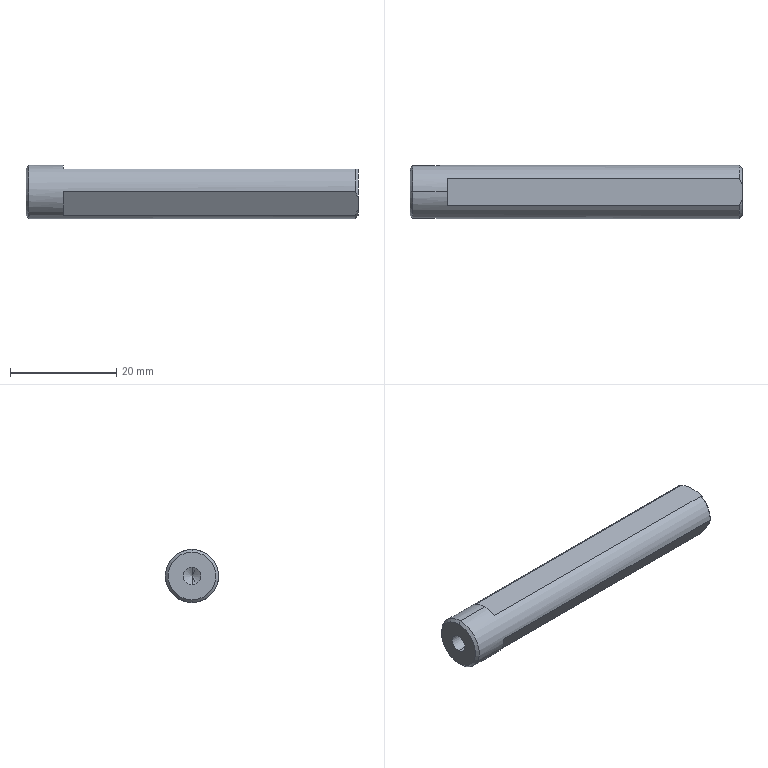Part | SolidWorks | features Chamfer 1, CirPattern 1, Extrusion 1, HoleWzd 1, ICE 1 | 1 solid | 19 faces | box 62.5 x 10 x 10 mm | volume 4365 mm3 | plane 8 | cone 7 | cylinder 4 | commonest cylinder face diameters 3.3 x2 10 x2
STEP:
#1=CARTESIAN_POINT('',(15.5,0.,-1.65));
#2=VERTEX_POINT('',#1);
#3=CARTESIAN_POINT('',(15.5,0.,1.65));
#4=VERTEX_POINT('',#3);
#5=CARTESIAN_POINT('',(15.5,0.,0.));
#6=DIRECTION('',(-1.,0.,0.));
#7=DIRECTION('',(0.,0.,1.));
#8=AXIS2_PLACEMENT_3D('',#5,#6,#7);
#9=CIRCLE('',#8,1.65);
#10=EDGE_CURVE('',#2,#4,#9,.T.);
#11=ORIENTED_EDGE('',*,*,#10,.F.);
#12=CARTESIAN_POINT('',(0.,0.,-1.65));
#13=VERTEX_POINT('',#12);
#14=CARTESIAN_POINT('',(0.,0.,-1.65));
#15=DIRECTION('',(-1.,0.,0.));
#16=VECTOR('',#15,1000.);
#17=LINE('',#14,#16);
#18=EDGE_CURVE('',#2,#13,#17,.T.);
#19=ORIENTED_EDGE('',*,*,#18,.T.);
#20=CARTESIAN_POINT('',(0.,0.,1.65));
#21=VERTEX_POINT('',#20);
#22=CARTESIAN_POINT('',(0.,0.,0.));
#23=DIRECTION('',(-1.,0.,0.));
#24=DIRECTION('',(0.,0.,1.));
#25=AXIS2_PLACEMENT_3D('',#22,#23,#24);
#26=CIRCLE('',#25,1.65);
#27=EDGE_CURVE('',#13,#21,#26,.T.);
#28=ORIENTED_EDGE('',*,*,#27,.T.);
#29=CARTESIAN_POINT('',(0.,0.,1.65));
#30=DIRECTION('',(-1.,0.,0.));
#31=VECTOR('',#30,1000.);
#32=LINE('',#29,#31);
#33=EDGE_CURVE('',#4,#21,#32,.T.);
#34=ORIENTED_EDGE('',*,*,#33,.F.);
#35=EDGE_LOOP('',(#11,#19,#28,#34));
#36=FACE_OUTER_BOUND('',#35,.T.);
#37=CARTESIAN_POINT('',(0.,0.,0.));
#38=DIRECTION('',(-1.,0.,0.));
#39=DIRECTION('',(0.,0.,1.));
#40=AXIS2_PLACEMENT_3D('',#37,#38,#39);
#41=CYLINDRICAL_SURFACE('',#40,1.65);
#42=ADVANCED_FACE('',(#36),#41,.F.);
#43=CARTESIAN_POINT('',(16.491,0.,0.));
#44=VERTEX_POINT('',#43);
#45=CARTESIAN_POINT('',(15.5,0.,1.65));
#46=DIRECTION('',(-0.515,0.,0.8572));
#47=VECTOR('',#46,1000.);
#48=LINE('',#45,#47);
#49=EDGE_CURVE('',#44,#4,#48,.T.);
#50=ORIENTED_EDGE('',*,*,#49,.F.);
#51=CARTESIAN_POINT('',(15.5,0.,-1.65));
#52=DIRECTION('',(-0.515,0.,-0.8572));
#53=VECTOR('',#52,1000.);
#54=LINE('',#51,#53);
#55=EDGE_CURVE('',#44,#2,#54,.T.);
#56=ORIENTED_EDGE('',*,*,#55,.T.);
#57=ORIENTED_EDGE('',*,*,#10,.T.);
#58=EDGE_LOOP('',(#50,#56,#57));
#59=FACE_OUTER_BOUND('',#58,.T.);
#60=CARTESIAN_POINT('',(15.5,0.,0.));
#61=DIRECTION('',(-1.,0.,0.));
#62=DIRECTION('',(0.,0.,1.));
#63=AXIS2_PLACEMENT_3D('',#60,#61,#62);
#64=CONICAL_SURFACE('',#63,1.65,1.03);
#65=ADVANCED_FACE('',(#59),#64,.F.);
#66=CARTESIAN_POINT('',(0.,0.,4.5));
#67=VERTEX_POINT('',#66);
#68=CARTESIAN_POINT('',(0.,0.,-4.5));
#69=VERTEX_POINT('',#68);
#70=CARTESIAN_POINT('',(0.,0.,0.));
#71=DIRECTION('',(-1.,0.,0.));
#72=DIRECTION('',(0.,0.,-1.));
#73=AXIS2_PLACEMENT_3D('',#70,#71,#72);
#74=CIRCLE('',#73,4.5);
#75=EDGE_CURVE('',#67,#69,#74,.T.);
#76=ORIENTED_EDGE('',*,*,#75,.F.);
#77=CARTESIAN_POINT('',(0.5,0.,5.));
#78=VERTEX_POINT('',#77);
#79=CARTESIAN_POINT('',(0.5,0.,5.));
#80=DIRECTION('',(0.7071,0.,0.7071));
#81=VECTOR('',#80,1000.);
#82=LINE('',#79,#81);
#83=EDGE_CURVE('',#67,#78,#82,.T.);
#84=ORIENTED_EDGE('',*,*,#83,.T.);
#85=CARTESIAN_POINT('',(0.5,0.,-5.));
#86=VERTEX_POINT('',#85);
#87=CARTESIAN_POINT('',(0.5,0.,0.));
#88=DIRECTION('',(1.,0.,0.));
#89=DIRECTION('',(0.,0.,-1.));
#90=AXIS2_PLACEMENT_3D('',#87,#88,#89);
#91=CIRCLE('',#90,5.);
#92=EDGE_CURVE('',#86,#78,#91,.T.);
#93=ORIENTED_EDGE('',*,*,#92,.F.);
#94=CARTESIAN_POINT('',(0.5,0.,-5.));
#95=DIRECTION('',(0.7071,0.,-0.7071));
#96=VECTOR('',#95,1000.);
#97=LINE('',#94,#96);
#98=EDGE_CURVE('',#69,#86,#97,.T.);
#99=ORIENTED_EDGE('',*,*,#98,.F.);
#100=EDGE_LOOP('',(#76,#84,#93,#99));
#101=FACE_OUTER_BOUND('',#100,.T.);
#102=CARTESIAN_POINT('',(0.5,0.,0.));
#103=DIRECTION('',(1.,0.,0.));
#104=DIRECTION('',(0.,0.,-1.));
#105=AXIS2_PLACEMENT_3D('',#102,#103,#104);
#106=CONICAL_SURFACE('',#105,5.,0.7854);
#107=ADVANCED_FACE('',(#101),#106,.T.);
#108=CARTESIAN_POINT('',(62.,2.448,-4.36));
#109=VERTEX_POINT('',#108);
#110=CARTESIAN_POINT('',(62.,0.,-5.));
#111=VERTEX_POINT('',#110);
#112=CARTESIAN_POINT('',(62.,0.,0.));
#113=DIRECTION('',(-1.,0.,0.));
#114=DIRECTION('',(0.,0.,-1.));
#115=AXIS2_PLACEMENT_3D('',#112,#113,#114);
#116=CIRCLE('',#115,5.);
#117=EDGE_CURVE('',#109,#111,#116,.T.);
#118=ORIENTED_EDGE('',*,*,#117,.T.);
#119=CARTESIAN_POINT('',(62.5,0.,-5.));
#120=DIRECTION('',(-1.,0.,0.));
#121=VECTOR('',#120,1000.);
#122=LINE('',#119,#121);
#123=EDGE_CURVE('',#111,#86,#122,.T.);
#124=ORIENTED_EDGE('',*,*,#123,.T.);
#125=ORIENTED_EDGE('',*,*,#92,.T.);
#126=CARTESIAN_POINT('',(7.,0.,5.));
#127=VERTEX_POINT('',#126);
#128=CARTESIAN_POINT('',(62.5,0.,5.));
#129=DIRECTION('',(-1.,0.,0.));
#130=VECTOR('',#129,1000.);
#131=LINE('',#128,#130);
#132=EDGE_CURVE('',#127,#78,#131,.T.);
#133=ORIENTED_EDGE('',*,*,#132,.F.);
#134=CARTESIAN_POINT('',(7.,2.551,4.3));
#135=VERTEX_POINT('',#134);
#136=CARTESIAN_POINT('',(7.,0.,0.));
#137=DIRECTION('',(1.,0.,0.));
#138=DIRECTION('',(0.,0.,-1.));
#139=AXIS2_PLACEMENT_3D('',#136,#137,#138);
#140=CIRCLE('',#139,5.);
#141=EDGE_CURVE('',#135,#127,#140,.T.);
#142=ORIENTED_EDGE('',*,*,#141,.F.);
#143=CARTESIAN_POINT('',(62.,2.551,4.3));
#144=VERTEX_POINT('',#143);
#145=CARTESIAN_POINT('',(62.5,2.551,4.3));
#146=DIRECTION('',(1.,0.,0.));
#147=VECTOR('',#146,1000.);
#148=LINE('',#145,#147);
#149=EDGE_CURVE('',#135,#144,#148,.T.);
#150=ORIENTED_EDGE('',*,*,#149,.T.);
#151=CARTESIAN_POINT('',(62.,5.,0.05964));
#152=VERTEX_POINT('',#151);
#153=CARTESIAN_POINT('',(62.,0.,0.));
#154=DIRECTION('',(-1.,0.,0.));
#155=DIRECTION('',(0.,0.,-1.));
#156=AXIS2_PLACEMENT_3D('',#153,#154,#155);
#157=CIRCLE('',#156,5.);
#158=EDGE_CURVE('',#144,#152,#157,.T.);
#159=ORIENTED_EDGE('',*,*,#158,.T.);
#160=CARTESIAN_POINT('',(7.,5.,0.05964));
#161=VERTEX_POINT('',#160);
#162=CARTESIAN_POINT('',(62.5,5.,0.05964));
#163=DIRECTION('',(-1.,0.,0.));
#164=VECTOR('',#163,1000.);
#165=LINE('',#162,#164);
#166=EDGE_CURVE('',#152,#161,#165,.T.);
#167=ORIENTED_EDGE('',*,*,#166,.T.);
#168=CARTESIAN_POINT('',(7.,2.448,-4.36));
#169=VERTEX_POINT('',#168);
#170=CARTESIAN_POINT('',(7.,0.,0.));
#171=DIRECTION('',(1.,0.,0.));
#172=DIRECTION('',(0.,0.,-1.));
#173=AXIS2_PLACEMENT_3D('',#170,#171,#172);
#174=CIRCLE('',#173,5.);
#175=EDGE_CURVE('',#169,#161,#174,.T.);
#176=ORIENTED_EDGE('',*,*,#175,.F.);
#177=CARTESIAN_POINT('',(62.5,2.448,-4.36));
#178=DIRECTION('',(1.,0.,0.));
#179=VECTOR('',#178,1000.);
#180=LINE('',#177,#179);
#181=EDGE_CURVE('',#169,#109,#180,.T.);
#182=ORIENTED_EDGE('',*,*,#181,.T.);
#183=EDGE_LOOP('',(#118,#124,#125,#133,#142,#150,#159,#167,#176,#182));
#184=FACE_OUTER_BOUND('',#183,.T.);
#185=CARTESIAN_POINT('',(62.5,0.,0.));
#186=DIRECTION('',(-1.,0.,0.));
#187=DIRECTION('',(0.,0.,1.));
#188=AXIS2_PLACEMENT_3D('',#185,#186,#187);
#189=CYLINDRICAL_SURFACE('',#188,5.);
#190=ADVANCED_FACE('',(#184),#189,.T.);
#191=CARTESIAN_POINT('',(62.,-2.448,-4.36));
#192=VERTEX_POINT('',#191);
#193=CARTESIAN_POINT('',(62.5,-3.061,-3.299));
#194=VERTEX_POINT('',#193);
#195=CARTESIAN_POINT('',(62.,-2.448,-4.36));
#196=CARTESIAN_POINT('',(62.201,-2.645,-4.019));
#197=CARTESIAN_POINT('',(62.374,-2.847,-3.668));
#198=CARTESIAN_POINT('',(62.5,-3.061,-3.299));
#199=B_SPLINE_CURVE_WITH_KNOTS('',3,(#195,#196,#197,#198),.UNSPECIFIED.,.F.,.F.,(4,4),(0.009242,0.01057),.UNSPECIFIED.);
#200=EDGE_CURVE('',#192,#194,#199,.T.);
#201=ORIENTED_EDGE('',*,*,#200,.F.);
#202=CARTESIAN_POINT('',(62.,0.,0.));
#203=DIRECTION('',(-1.,0.,0.));
#204=DIRECTION('',(0.,0.,-1.));
#205=AXIS2_PLACEMENT_3D('',#202,#203,#204);
#206=CIRCLE('',#205,5.);
#207=EDGE_CURVE('',#111,#192,#206,.T.);
#208=ORIENTED_EDGE('',*,*,#207,.F.);
#209=ORIENTED_EDGE('',*,*,#117,.F.);
#210=CARTESIAN_POINT('',(62.5,3.061,-3.299));
#211=VERTEX_POINT('',#210);
#212=CARTESIAN_POINT('',(62.5,3.061,-3.299));
#213=CARTESIAN_POINT('',(62.438,2.955,-3.482));
#214=CARTESIAN_POINT('',(62.362,2.85,-3.664));
#215=CARTESIAN_POINT('',(62.193,2.645,-4.018));
#216=CARTESIAN_POINT('',(62.1,2.546,-4.191));
#217=CARTESIAN_POINT('',(62.,2.448,-4.36));
#218=B_SPLINE_CURVE_WITH_KNOTS('',3,(#212,#213,#214,#215,#216,#217),.UNSPECIFIED.,.F.,.F.,(4,2,4),(0.01336,0.01402,0.01468),.UNSPECIFIED.);
#219=EDGE_CURVE('',#211,#109,#218,.T.);
#220=ORIENTED_EDGE('',*,*,#219,.F.);
#221=CARTESIAN_POINT('',(62.5,0.,0.));
#222=DIRECTION('',(1.,0.,0.));
#223=DIRECTION('',(0.,0.,-1.));
#224=AXIS2_PLACEMENT_3D('',#221,#222,#223);
#225=CIRCLE('',#224,4.5);
#226=EDGE_CURVE('',#194,#211,#225,.T.);
#227=ORIENTED_EDGE('',*,*,#226,.F.);
#228=EDGE_LOOP('',(#201,#208,#209,#220,#227));
#229=FACE_OUTER_BOUND('',#228,.T.);
#230=CARTESIAN_POINT('',(62.5,0.,0.));
#231=DIRECTION('',(-1.,0.,0.));
#232=DIRECTION('',(0.,0.,1.));
#233=AXIS2_PLACEMENT_3D('',#230,#231,#232);
#234=CONICAL_SURFACE('',#233,4.5,0.7854);
#235=ADVANCED_FACE('',(#229),#234,.T.);
#236=CARTESIAN_POINT('',(62.5,4.387,-1.001));
#237=VERTEX_POINT('',#236);
#238=CARTESIAN_POINT('',(62.,5.,0.05964));
#239=CARTESIAN_POINT('',(62.201,4.803,-0.2807));
#240=CARTESIAN_POINT('',(62.374,4.601,-0.6315));
#241=CARTESIAN_POINT('',(62.5,4.387,-1.001));
#242=B_SPLINE_CURVE_WITH_KNOTS('',3,(#238,#239,#240,#241),.UNSPECIFIED.,.F.,.F.,(4,4),(0.00934,0.01066),.UNSPECIFIED.);
#243=EDGE_CURVE('',#152,#237,#242,.T.);
#244=ORIENTED_EDGE('',*,*,#243,.F.);
#245=ORIENTED_EDGE('',*,*,#158,.F.);
#246=CARTESIAN_POINT('',(62.5,1.327,4.3));
#247=VERTEX_POINT('',#246);
#248=CARTESIAN_POINT('',(62.5,1.327,4.3));
#249=CARTESIAN_POINT('',(62.437,1.539,4.3));
#250=CARTESIAN_POINT('',(62.362,1.749,4.3));
#251=CARTESIAN_POINT('',(62.193,2.157,4.3));
#252=CARTESIAN_POINT('',(62.1,2.356,4.3));
#253=CARTESIAN_POINT('',(62.,2.551,4.3));
#254=B_SPLINE_CURVE_WITH_KNOTS('',3,(#248,#249,#250,#251,#252,#253),.UNSPECIFIED.,.F.,.F.,(4,2,4),(0.01372,0.01438,0.01504),.UNSPECIFIED.);
#255=EDGE_CURVE('',#247,#144,#254,.T.);
#256=ORIENTED_EDGE('',*,*,#255,.F.);
#257=CARTESIAN_POINT('',(62.5,0.,0.));
#258=DIRECTION('',(1.,0.,0.));
#259=DIRECTION('',(0.,0.,-1.));
#260=AXIS2_PLACEMENT_3D('',#257,#258,#259);
#261=CIRCLE('',#260,4.5);
#262=EDGE_CURVE('',#237,#247,#261,.T.);
#263=ORIENTED_EDGE('',*,*,#262,.F.);
#264=EDGE_LOOP('',(#244,#245,#256,#263));
#265=FACE_OUTER_BOUND('',#264,.T.);
#266=CARTESIAN_POINT('',(62.5,0.,0.));
#267=DIRECTION('',(-1.,0.,0.));
#268=DIRECTION('',(0.,0.,1.));
#269=AXIS2_PLACEMENT_3D('',#266,#267,#268);
#270=CONICAL_SURFACE('',#269,4.5,0.7854);
#271=ADVANCED_FACE('',(#265),#270,.T.);
#272=ORIENTED_EDGE('',*,*,#123,.F.);
#273=ORIENTED_EDGE('',*,*,#207,.T.);
#274=CARTESIAN_POINT('',(7.,-2.448,-4.36));
#275=VERTEX_POINT('',#274);
#276=CARTESIAN_POINT('',(62.5,-2.448,-4.36));
#277=DIRECTION('',(-1.,0.,0.));
#278=VECTOR('',#277,1000.);
#279=LINE('',#276,#278);
#280=EDGE_CURVE('',#192,#275,#279,.T.);
#281=ORIENTED_EDGE('',*,*,#280,.T.);
#282=CARTESIAN_POINT('',(7.,-5.,0.05964));
#283=VERTEX_POINT('',#282);
#284=CARTESIAN_POINT('',(7.,0.,0.));
#285=DIRECTION('',(1.,0.,0.));
#286=DIRECTION('',(0.,0.,-1.));
#287=AXIS2_PLACEMENT_3D('',#284,#285,#286);
#288=CIRCLE('',#287,5.);
#289=EDGE_CURVE('',#283,#275,#288,.T.);
#290=ORIENTED_EDGE('',*,*,#289,.F.);
#291=CARTESIAN_POINT('',(62.,-5.,0.05964));
#292=VERTEX_POINT('',#291);
#293=CARTESIAN_POINT('',(62.5,-5.,0.05964));
#294=DIRECTION('',(1.,0.,0.));
#295=VECTOR('',#294,1000.);
#296=LINE('',#293,#295);
#297=EDGE_CURVE('',#283,#292,#296,.T.);
#298=ORIENTED_EDGE('',*,*,#297,.T.);
#299=CARTESIAN_POINT('',(62.,-2.551,4.3));
#300=VERTEX_POINT('',#299);
#301=CARTESIAN_POINT('',(62.,0.,0.));
#302=DIRECTION('',(-1.,0.,0.));
#303=DIRECTION('',(0.,0.,-1.));
#304=AXIS2_PLACEMENT_3D('',#301,#302,#303);
#305=CIRCLE('',#304,5.);
#306=EDGE_CURVE('',#292,#300,#305,.T.);
#307=ORIENTED_EDGE('',*,*,#306,.T.);
#308=CARTESIAN_POINT('',(7.,-2.551,4.3));
#309=VERTEX_POINT('',#308);
#310=CARTESIAN_POINT('',(62.5,-2.551,4.3));
#311=DIRECTION('',(-1.,0.,0.));
#312=VECTOR('',#311,1000.);
#313=LINE('',#310,#312);
#314=EDGE_CURVE('',#300,#309,#313,.T.);
#315=ORIENTED_EDGE('',*,*,#314,.T.);
#316=CARTESIAN_POINT('',(7.,0.,0.));
#317=DIRECTION('',(1.,0.,0.));
#318=DIRECTION('',(0.,0.,-1.));
#319=AXIS2_PLACEMENT_3D('',#316,#317,#318);
#320=CIRCLE('',#319,5.);
#321=EDGE_CURVE('',#127,#309,#320,.T.);
#322=ORIENTED_EDGE('',*,*,#321,.F.);
#323=ORIENTED_EDGE('',*,*,#132,.T.);
#324=CARTESIAN_POINT('',(0.5,0.,0.));
#325=DIRECTION('',(1.,0.,0.));
#326=DIRECTION('',(0.,0.,-1.));
#327=AXIS2_PLACEMENT_3D('',#324,#325,#326);
#328=CIRCLE('',#327,5.);
#329=EDGE_CURVE('',#78,#86,#328,.T.);
#330=ORIENTED_EDGE('',*,*,#329,.T.);
#331=EDGE_LOOP('',(#272,#273,#281,#290,#298,#307,#315,#322,#323,#330));
#332=FACE_OUTER_BOUND('',#331,.T.);
#333=CARTESIAN_POINT('',(62.5,0.,0.));
#334=DIRECTION('',(-1.,0.,0.));
#335=DIRECTION('',(0.,0.,1.));
#336=AXIS2_PLACEMENT_3D('',#333,#334,#335);
#337=CYLINDRICAL_SURFACE('',#336,5.);
#338=ADVANCED_FACE('',(#332),#337,.T.);
#339=CARTESIAN_POINT('',(62.5,-4.387,-1.001));
#340=VERTEX_POINT('',#339);
#341=CARTESIAN_POINT('',(62.5,-6.886,3.326));
#342=DIRECTION('',(0.,-0.5,0.866));
#343=VECTOR('',#342,1000.);
#344=LINE('',#341,#343);
#345=EDGE_CURVE('',#194,#340,#344,.T.);
#346=ORIENTED_EDGE('',*,*,#345,.F.);
#347=ORIENTED_EDGE('',*,*,#226,.T.);
#348=CARTESIAN_POINT('',(62.5,0.5621,-7.626));
#349=DIRECTION('',(0.,-0.5,-0.866));
#350=VECTOR('',#349,1000.);
#351=LINE('',#348,#350);
#352=EDGE_CURVE('',#237,#211,#351,.T.);
#353=ORIENTED_EDGE('',*,*,#352,.F.);
#354=ORIENTED_EDGE('',*,*,#262,.T.);
#355=CARTESIAN_POINT('',(62.5,-1.327,4.3));
#356=VERTEX_POINT('',#355);
#357=CARTESIAN_POINT('',(62.5,6.324,4.3));
#358=DIRECTION('',(0.,1.,0.));
#359=VECTOR('',#358,1000.);
#360=LINE('',#357,#359);
#361=EDGE_CURVE('',#356,#247,#360,.T.);
#362=ORIENTED_EDGE('',*,*,#361,.F.);
#363=CARTESIAN_POINT('',(62.5,0.,0.));
#364=DIRECTION('',(1.,0.,0.));
#365=DIRECTION('',(0.,0.,-1.));
#366=AXIS2_PLACEMENT_3D('',#363,#364,#365);
#367=CIRCLE('',#366,4.5);
#368=EDGE_CURVE('',#356,#340,#367,.T.);
#369=ORIENTED_EDGE('',*,*,#368,.T.);
#370=EDGE_LOOP('',(#346,#347,#353,#354,#362,#369));
#371=FACE_OUTER_BOUND('',#370,.T.);
#372=CARTESIAN_POINT('',(62.5,0.,0.));
#373=DIRECTION('',(1.,0.,0.));
#374=DIRECTION('',(0.,0.,-1.));
#375=AXIS2_PLACEMENT_3D('',#372,#373,#374);
#376=PLANE('',#375);
#377=ADVANCED_FACE('',(#371),#376,.T.);
#378=CARTESIAN_POINT('',(0.,0.,0.));
#379=DIRECTION('',(-1.,0.,0.));
#380=DIRECTION('',(0.,0.,1.));
#381=AXIS2_PLACEMENT_3D('',#378,#379,#380);
#382=CIRCLE('',#381,1.65);
#383=EDGE_CURVE('',#21,#13,#382,.T.);
#384=ORIENTED_EDGE('',*,*,#383,.F.);
#385=ORIENTED_EDGE('',*,*,#27,.F.);
#386=EDGE_LOOP('',(#384,#385));
#387=FACE_BOUND('',#386,.T.);
#388=CARTESIAN_POINT('',(0.,0.,0.));
#389=DIRECTION('',(-1.,0.,0.));
#390=DIRECTION('',(0.,0.,-1.));
#391=AXIS2_PLACEMENT_3D('',#388,#389,#390);
#392=CIRCLE('',#391,4.5);
#393=EDGE_CURVE('',#69,#67,#392,.T.);
#394=ORIENTED_EDGE('',*,*,#393,.T.);
#395=ORIENTED_EDGE('',*,*,#75,.T.);
#396=EDGE_LOOP('',(#394,#395));
#397=FACE_OUTER_BOUND('',#396,.T.);
#398=CARTESIAN_POINT('',(0.,0.,0.));
#399=DIRECTION('',(1.,0.,0.));
#400=DIRECTION('',(0.,0.,-1.));
#401=AXIS2_PLACEMENT_3D('',#398,#399,#400);
#402=PLANE('',#401);
#403=ADVANCED_FACE('',(#387,#397),#402,.F.);
#404=ORIENTED_EDGE('',*,*,#83,.F.);
#405=ORIENTED_EDGE('',*,*,#393,.F.);
#406=ORIENTED_EDGE('',*,*,#98,.T.);
#407=ORIENTED_EDGE('',*,*,#329,.F.);
#408=EDGE_LOOP('',(#404,#405,#406,#407));
#409=FACE_OUTER_BOUND('',#408,.T.);
#410=CARTESIAN_POINT('',(0.5,0.,0.));
#411=DIRECTION('',(1.,0.,0.));
#412=DIRECTION('',(0.,0.,-1.));
#413=AXIS2_PLACEMENT_3D('',#410,#411,#412);
#414=CONICAL_SURFACE('',#413,5.,0.7854);
#415=ADVANCED_FACE('',(#409),#414,.T.);
#416=CARTESIAN_POINT('',(62.5,-4.387,-1.001));
#417=CARTESIAN_POINT('',(62.438,-4.493,-0.8177));
#418=CARTESIAN_POINT('',(62.362,-4.598,-0.6358));
#419=CARTESIAN_POINT('',(62.193,-4.802,-0.2819));
#420=CARTESIAN_POINT('',(62.1,-4.902,-0.1094));
#421=CARTESIAN_POINT('',(62.,-5.,0.05964));
#422=B_SPLINE_CURVE_WITH_KNOTS('',3,(#416,#417,#418,#419,#420,#421),.UNSPECIFIED.,.F.,.F.,(4,2,4),(0.01326,0.01392,0.01459),.UNSPECIFIED.);
#423=EDGE_CURVE('',#340,#292,#422,.T.);
#424=ORIENTED_EDGE('',*,*,#423,.F.);
#425=ORIENTED_EDGE('',*,*,#368,.F.);
#426=CARTESIAN_POINT('',(62.,-2.551,4.3));
#427=CARTESIAN_POINT('',(62.2,-2.159,4.3));
#428=CARTESIAN_POINT('',(62.375,-1.752,4.3));
#429=CARTESIAN_POINT('',(62.5,-1.327,4.3));
#430=B_SPLINE_CURVE_WITH_KNOTS('',3,(#426,#427,#428,#429),.UNSPECIFIED.,.F.,.F.,(4,4),(0.009698,0.01102),.UNSPECIFIED.);
#431=EDGE_CURVE('',#300,#356,#430,.T.);
#432=ORIENTED_EDGE('',*,*,#431,.F.);
#433=ORIENTED_EDGE('',*,*,#306,.F.);
#434=EDGE_LOOP('',(#424,#425,#432,#433));
#435=FACE_OUTER_BOUND('',#434,.T.);
#436=CARTESIAN_POINT('',(62.5,0.,0.));
#437=DIRECTION('',(-1.,0.,0.));
#438=DIRECTION('',(0.,0.,1.));
#439=AXIS2_PLACEMENT_3D('',#436,#437,#438);
#440=CONICAL_SURFACE('',#439,4.5,0.7854);
#441=ADVANCED_FACE('',(#435),#440,.T.);
#442=ORIENTED_EDGE('',*,*,#141,.T.);
#443=ORIENTED_EDGE('',*,*,#321,.T.);
#444=CARTESIAN_POINT('',(7.,6.324,4.3));
#445=DIRECTION('',(0.,1.,0.));
#446=VECTOR('',#445,1000.);
#447=LINE('',#444,#446);
#448=EDGE_CURVE('',#309,#135,#447,.T.);
#449=ORIENTED_EDGE('',*,*,#448,.T.);
#450=EDGE_LOOP('',(#442,#443,#449));
#451=FACE_OUTER_BOUND('',#450,.T.);
#452=CARTESIAN_POINT('',(7.,0.,0.));
#453=DIRECTION('',(1.,0.,0.));
#454=DIRECTION('',(0.,0.,-1.));
#455=AXIS2_PLACEMENT_3D('',#452,#453,#454);
#456=PLANE('',#455);
#457=ADVANCED_FACE('',(#451),#456,.T.);
#458=ORIENTED_EDGE('',*,*,#431,.T.);
#459=ORIENTED_EDGE('',*,*,#361,.T.);
#460=ORIENTED_EDGE('',*,*,#255,.T.);
#461=ORIENTED_EDGE('',*,*,#149,.F.);
#462=ORIENTED_EDGE('',*,*,#448,.F.);
#463=ORIENTED_EDGE('',*,*,#314,.F.);
#464=EDGE_LOOP('',(#458,#459,#460,#461,#462,#463));
#465=FACE_OUTER_BOUND('',#464,.T.);
#466=CARTESIAN_POINT('',(7.,6.324,4.3));
#467=DIRECTION('',(0.,0.,-1.));
#468=DIRECTION('',(0.,1.,0.));
#469=AXIS2_PLACEMENT_3D('',#466,#467,#468);
#470=PLANE('',#469);
#471=ADVANCED_FACE('',(#465),#470,.F.);
#472=ORIENTED_EDGE('',*,*,#175,.T.);
#473=CARTESIAN_POINT('',(7.,0.5621,-7.626));
#474=DIRECTION('',(0.,-0.5,-0.866));
#475=VECTOR('',#474,1000.);
#476=LINE('',#473,#475);
#477=EDGE_CURVE('',#161,#169,#476,.T.);
#478=ORIENTED_EDGE('',*,*,#477,.T.);
#479=EDGE_LOOP('',(#472,#478));
#480=FACE_OUTER_BOUND('',#479,.T.);
#481=CARTESIAN_POINT('',(7.,0.,0.));
#482=DIRECTION('',(1.,0.,0.));
#483=DIRECTION('',(0.,-0.866,0.5));
#484=AXIS2_PLACEMENT_3D('',#481,#482,#483);
#485=PLANE('',#484);
#486=ADVANCED_FACE('',(#480),#485,.T.);
#487=ORIENTED_EDGE('',*,*,#243,.T.);
#488=ORIENTED_EDGE('',*,*,#352,.T.);
#489=ORIENTED_EDGE('',*,*,#219,.T.);
#490=ORIENTED_EDGE('',*,*,#181,.F.);
#491=ORIENTED_EDGE('',*,*,#477,.F.);
#492=ORIENTED_EDGE('',*,*,#166,.F.);
#493=EDGE_LOOP('',(#487,#488,#489,#490,#491,#492));
#494=FACE_OUTER_BOUND('',#493,.T.);
#495=CARTESIAN_POINT('',(7.,0.5621,-7.626));
#496=DIRECTION('',(0.,-0.866,0.5));
#497=DIRECTION('',(0.,-0.5,-0.866));
#498=AXIS2_PLACEMENT_3D('',#495,#496,#497);
#499=PLANE('',#498);
#500=ADVANCED_FACE('',(#494),#499,.F.);
#501=ORIENTED_EDGE('',*,*,#289,.T.);
#502=CARTESIAN_POINT('',(7.,-6.886,3.326));
#503=DIRECTION('',(0.,-0.5,0.866));
#504=VECTOR('',#503,1000.);
#505=LINE('',#502,#504);
#506=EDGE_CURVE('',#275,#283,#505,.T.);
#507=ORIENTED_EDGE('',*,*,#506,.T.);
#508=EDGE_LOOP('',(#501,#507));
#509=FACE_OUTER_BOUND('',#508,.T.);
#510=CARTESIAN_POINT('',(7.,0.,0.));
#511=DIRECTION('',(1.,0.,0.));
#512=DIRECTION('',(0.,0.866,0.5));
#513=AXIS2_PLACEMENT_3D('',#510,#511,#512);
#514=PLANE('',#513);
#515=ADVANCED_FACE('',(#509),#514,.T.);
#516=ORIENTED_EDGE('',*,*,#200,.T.);
#517=ORIENTED_EDGE('',*,*,#345,.T.);
#518=ORIENTED_EDGE('',*,*,#423,.T.);
#519=ORIENTED_EDGE('',*,*,#297,.F.);
#520=ORIENTED_EDGE('',*,*,#506,.F.);
#521=ORIENTED_EDGE('',*,*,#280,.F.);
#522=EDGE_LOOP('',(#516,#517,#518,#519,#520,#521));
#523=FACE_OUTER_BOUND('',#522,.T.);
#524=CARTESIAN_POINT('',(7.,-6.886,3.326));
#525=DIRECTION('',(0.,0.866,0.5));
#526=DIRECTION('',(0.,-0.5,0.866));
#527=AXIS2_PLACEMENT_3D('',#524,#525,#526);
#528=PLANE('',#527);
#529=ADVANCED_FACE('',(#523),#528,.F.);
#530=ORIENTED_EDGE('',*,*,#55,.F.);
#531=ORIENTED_EDGE('',*,*,#49,.T.);
#532=CARTESIAN_POINT('',(15.5,0.,0.));
#533=DIRECTION('',(-1.,0.,0.));
#534=DIRECTION('',(0.,0.,1.));
#535=AXIS2_PLACEMENT_3D('',#532,#533,#534);
#536=CIRCLE('',#535,1.65);
#537=EDGE_CURVE('',#4,#2,#536,.T.);
#538=ORIENTED_EDGE('',*,*,#537,.T.);
#539=EDGE_LOOP('',(#530,#531,#538));
#540=FACE_OUTER_BOUND('',#539,.T.);
#541=CARTESIAN_POINT('',(15.5,0.,0.));
#542=DIRECTION('',(-1.,0.,0.));
#543=DIRECTION('',(0.,0.,1.));
#544=AXIS2_PLACEMENT_3D('',#541,#542,#543);
#545=CONICAL_SURFACE('',#544,1.65,1.03);
#546=ADVANCED_FACE('',(#540),#545,.F.);
#547=ORIENTED_EDGE('',*,*,#18,.F.);
#548=ORIENTED_EDGE('',*,*,#537,.F.);
#549=ORIENTED_EDGE('',*,*,#33,.T.);
#550=ORIENTED_EDGE('',*,*,#383,.T.);
#551=EDGE_LOOP('',(#547,#548,#549,#550));
#552=FACE_OUTER_BOUND('',#551,.T.);
#553=CARTESIAN_POINT('',(0.,0.,0.));
#554=DIRECTION('',(-1.,0.,0.));
#555=DIRECTION('',(0.,0.,1.));
#556=AXIS2_PLACEMENT_3D('',#553,#554,#555);
#557=CYLINDRICAL_SURFACE('',#556,1.65);
#558=ADVANCED_FACE('',(#552),#557,.F.);
#559=CLOSED_SHELL('',(#42,#65,#107,#190,#235,#271,#338,#377,#403,#415,#441,#457,#471,#486,#500,#515,#529,#546,#558));
#560=MANIFOLD_SOLID_BREP('',#559);
#561=CARTESIAN_POINT('',(0.,0.,0.));
#562=DIRECTION('',(0.,0.,1.));
#563=DIRECTION('',(1.,0.,0.));
#564=AXIS2_PLACEMENT_3D('',#561,#562,#563);
#565=(LENGTH_UNIT()NAMED_UNIT(*)SI_UNIT(.MILLI.,.METRE.));
#566=UNCERTAINTY_MEASURE_WITH_UNIT(LENGTH_MEASURE(0.00001),#565,'','');
#567=(NAMED_UNIT(*)PLANE_ANGLE_UNIT()SI_UNIT($,.RADIAN.));
#568=(NAMED_UNIT(*)SI_UNIT($,.STERADIAN.)SOLID_ANGLE_UNIT());
#569=(GEOMETRIC_REPRESENTATION_CONTEXT(3)GLOBAL_UNCERTAINTY_ASSIGNED_CONTEXT((#566))GLOBAL_UNIT_ASSIGNED_CONTEXT((#565,#567,#568))REPRESENTATION_CONTEXT('',''));
#570=ADVANCED_BREP_SHAPE_REPRESENTATION('',(#560,#564),#569);